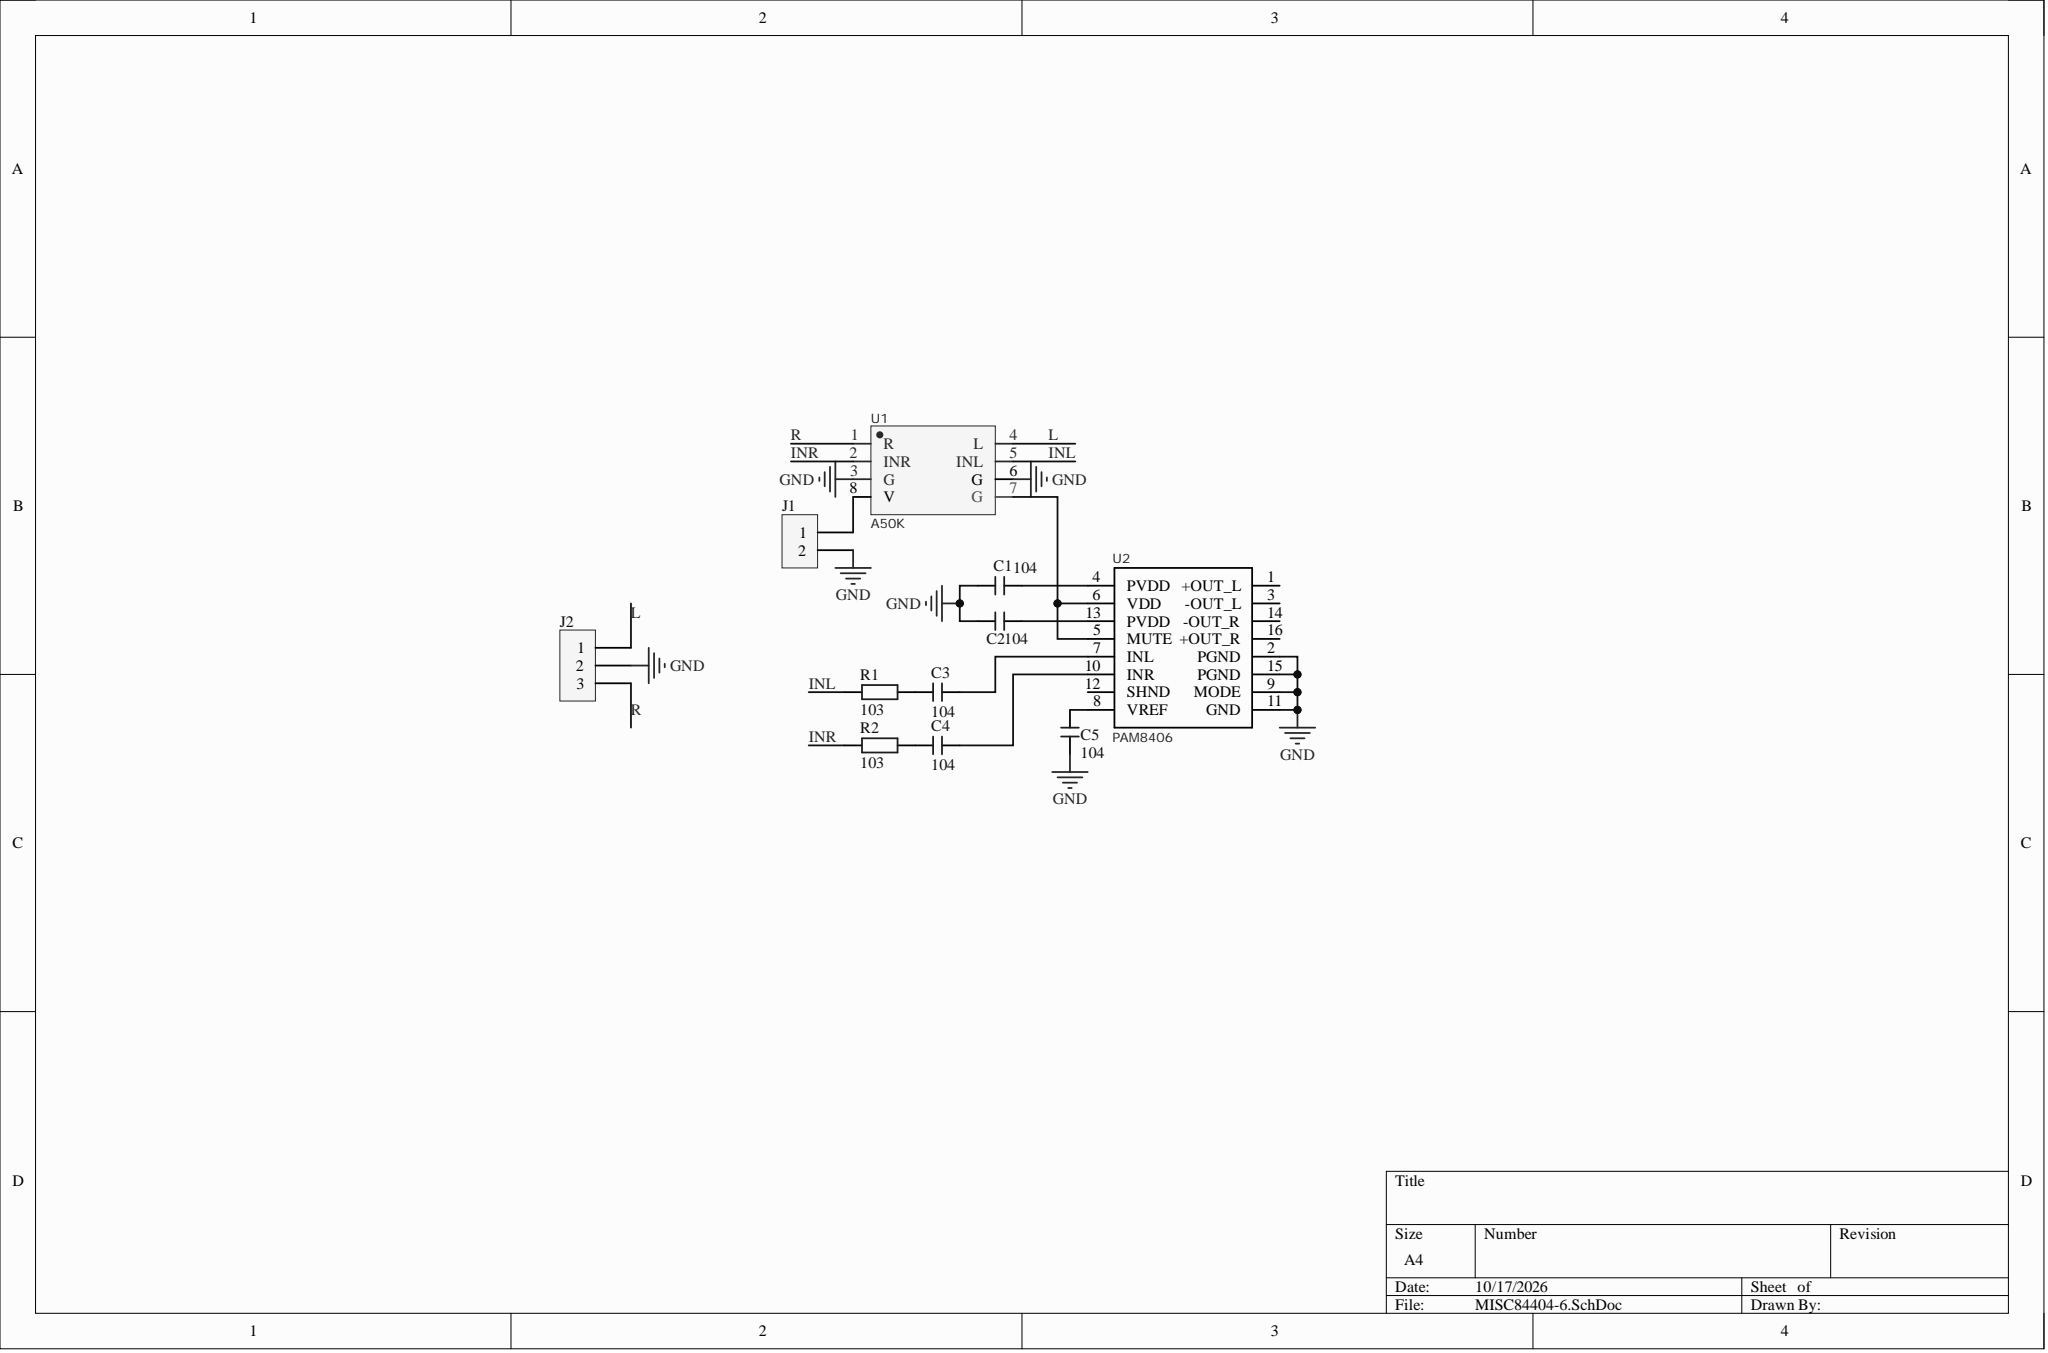Circuit board | Altium Designer | 11 parts | 14 nets
Bill of materials:
Comment,Description,Designator,Footprint,LibRef,Quantity
"104","Chip capacitor","C1, C2, C3, C4, C5","C 0805_L","C","5"
"Female HDR1X2","","J1","Fe-HDR1X2/2.54-S","Female HDR1X2","1"
"Female HDR1X3","","J2","Fe-HDR1X3/2.54-S","Female HDR1X3","1"
"103","Chip resistor","R1, R2","R 0805_L","R","2"
"A50K","","U1","SOP-8_L7.0-W7.0-P1.27-LS8.6-BL","GZP6832A010115KPA50KL","1"
"PAM8406","","U2","SOP16","PAM8406","1"
Netlist (Protel format):
[
C1
C 0805_L
104



]
[
C2
C 0805_L
104



]
[
C3
C 0805_L
104



]
[
C4
C 0805_L
104



]
[
C5
C 0805_L
104



]
[
J1
Fe-HDR1X2/2.54-S
Female HDR1X2



]
[
J2
Fe-HDR1X3/2.54-S
Female HDR1X3



]
[
R1
R 0805_L
103



]
[
R2
R 0805_L
103



]
[
U1
SOP-8_L7.0-W7.0-P1.27-LS8.6-BL
A50K



]
[
U2
SOP16
PAM8406



]
(
R
J2-3
U1-1
)
(
NetU1_7
U1-7
U2-5
U2-6
)
(
NetJ1_1
J1-1
U1-8
)
(
NetC5_2
C5-2
U2-8
)
(
NetC4_2
C4-2
R2-2
)
(
NetC4_1
C4-1
U2-10
)
(
NetC3_2
C3-2
R1-2
)
(
NetC3_1
C3-1
U2-7
)
(
NetC2_2
C2-2
U2-13
)
(
NetC1_2
C1-2
U2-4
)
(
L
J2-1
U1-4
)
(
INR
R2-1
U1-2
)
(
INL
R1-1
U1-5
)
(
GND
C1-1
C2-1
C5-1
J1-2
J2-2
U1-3
U1-6
U2-2
U2-9
U2-11
U2-15
)